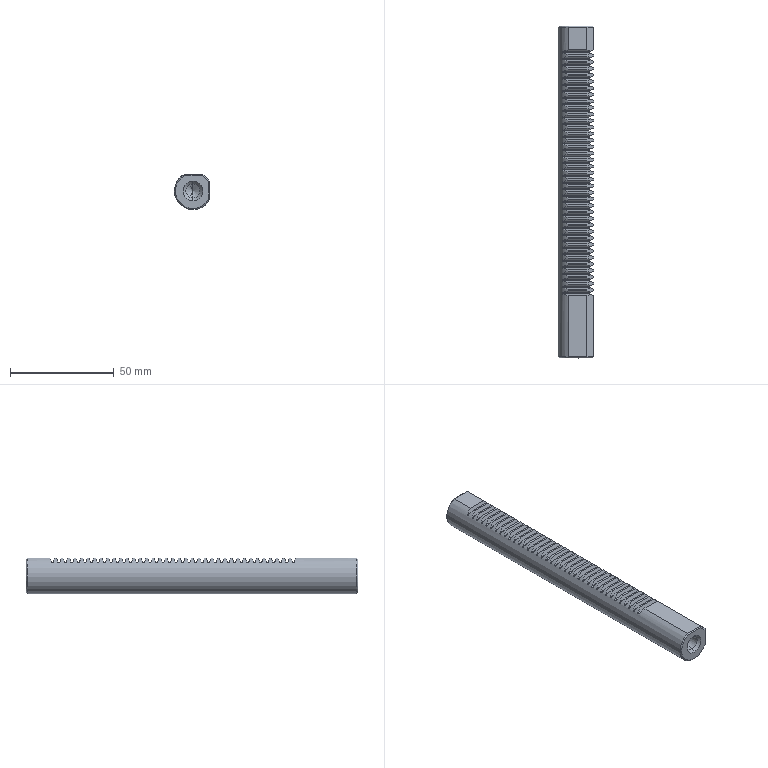Part | SolidWorks | features BaseBody 1 | 1 solid | 516 faces | box 17 x 160 x 17 mm | volume 35318 mm3 | plane 353 | cylinder 156 | cone 7 | commonest cylinder face diameters 0.76 x152 6.8 x2 18 x2